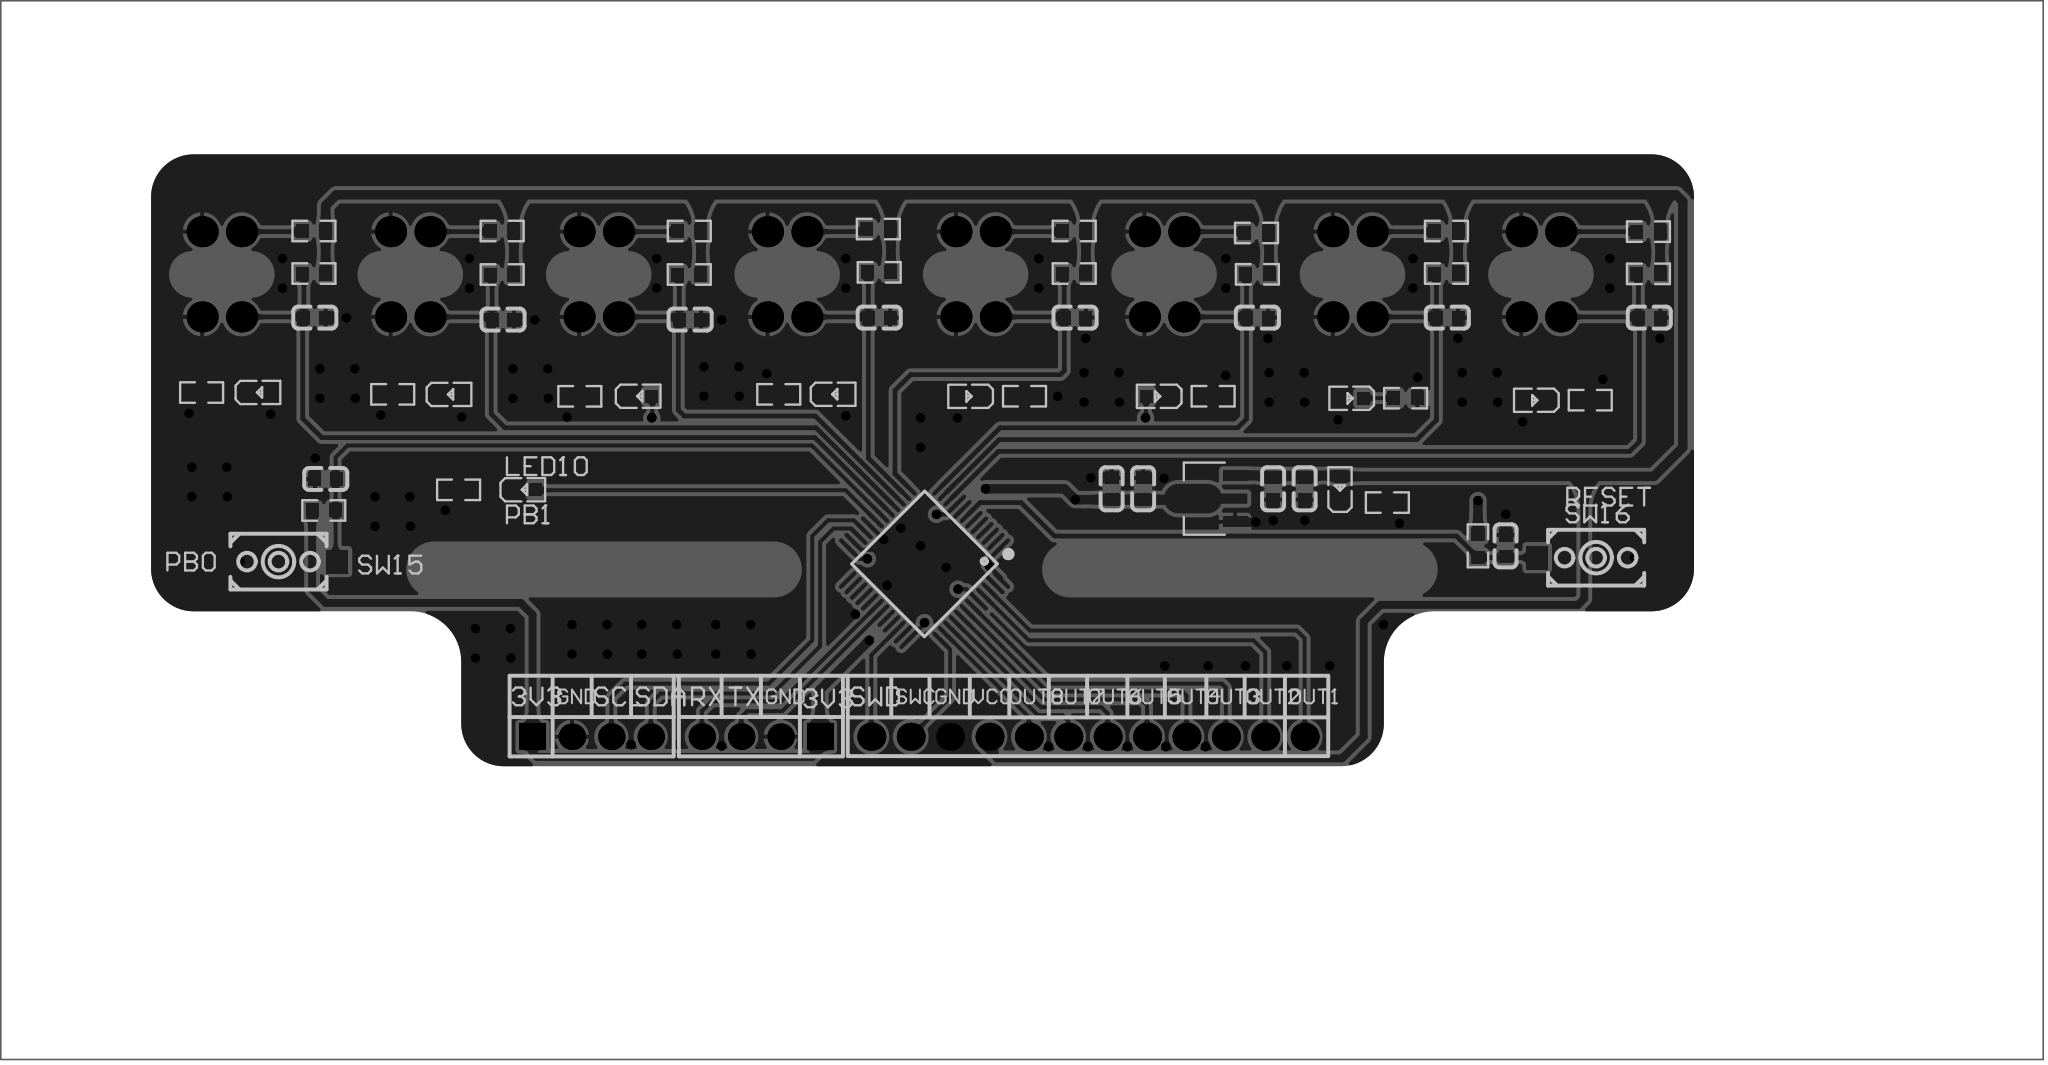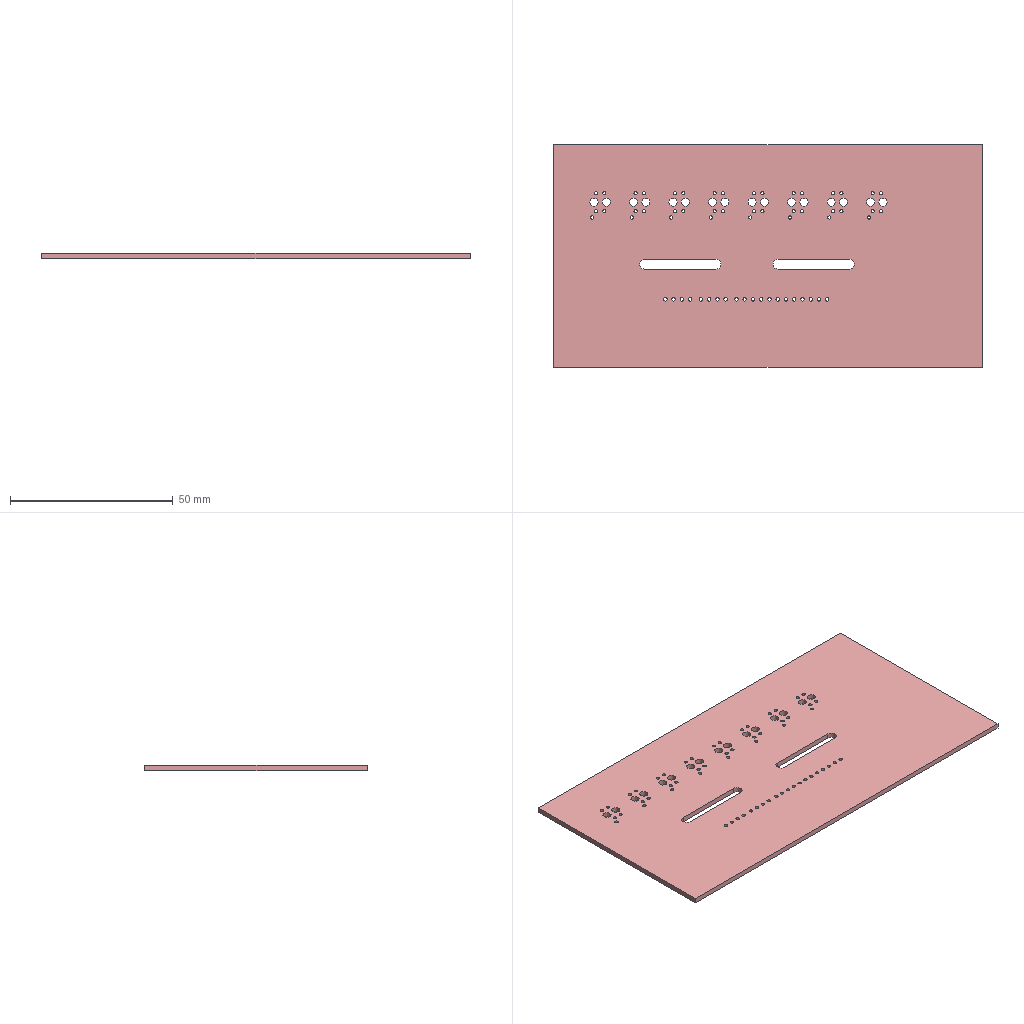Circuit board layout | Altium Designer | box 131.7 x 68.3 x 1.6 mm
Layer stack:
# Altium Designer layer stack of  (unit mm; dielectric type: 0 none, 1 core, 2 prepreg, 3 surface material)
index,name,kind,layer,copper_thickness_mm,dielectric_type,dielectric_thickness_mm,dielectric_material,dielectric_constant
0,Top Paste Mask Layer,other,,,,,,
1,Top Silkscreen Layer,other,,,,,,
2,Top Solder Mask Layer,dielectric,,,3,0.01,,3.3
3,Top Layer,copper,Top Layer,0.035,,,,
4,Dielectric1,dielectric,,,3,1.51,FR4,4.5
5,Bottom Layer,copper,Bottom Layer,0.035,,,,
6,Bottom Solder Mask Layer,dielectric,,,3,0.01,,3.3
7,Bottom Silkscreen Layer,other,,,,,,
8,Bottom Paste Mask Layer,other,,,,,,
# drill layer pairs: low layer,high layer
drill_pair,Top Layer,Bottom Layer
Part placement:
Designator,Comment,Layer,Footprint,Center-X(mm),Center-Y(mm),Rotation
CGQ1,TCRT5000L,BottomLayer,OPTO-TH_TCRT5000L,169.164,120.523,90
CGQ2,TCRT5000L,BottomLayer,OPTO-TH_TCRT5000L,157.013,120.523,90
CGQ3,TCRT5000L,BottomLayer,OPTO-TH_TCRT5000L,144.862,120.523,90
CGQ4,TCRT5000L,BottomLayer,OPTO-TH_TCRT5000L,132.711,120.523,90
CGQ5,TCRT5000L,BottomLayer,OPTO-TH_TCRT5000L,120.559,120.523,90
CGQ6,TCRT5000L,BottomLayer,OPTO-TH_TCRT5000L,108.408,120.523,90
CGQ7,TCRT5000L,BottomLayer,OPTO-TH_TCRT5000L,96.257,120.523,90
CGQ8,TCRT5000L,BottomLayer,OPTO-TH_TCRT5000L,84.106,120.523,90
H1,,TopLayer,HDR-TH_12P-P2.54-V-F,139.954,90.678,180
H2,,TopLayer,HDR-TH_4P-P2.54-V-F,107.95,90.678,0
H3,,TopLayer,HDR-TH_4P-P2.54-V-F,118.864,90.683,180
LED1,NCD0603R1,TopLayer,LED0603-RD_RED,168.815,112.4,180
LED2,NCD0603R1,TopLayer,LED0603-RD_RED,156.91,112.527,180
LED3,NCD0603R1,TopLayer,LED0603-RD_RED,144.496,112.654,180
LED4,NCD0603R1,TopLayer,LED0603-RD_RED,132.336,112.654,180
LED5,NCD0603R1,TopLayer,LED0603-RD_RED,123.571,112.776,0
LED6,NCD0603R1,TopLayer,LED0603-RD_RED,110.998,112.649,0
LED7,NCD0603R1,TopLayer,LED0603-RD_RED,98.802,112.765,0
LED8,NCD0603R1,TopLayer,LED0603-RD_RED,86.483,112.892,0
LED9,NCD0603R1,TopLayer,LED0603-RD_RED,156.21,106.68,90
LED10,NCD0603R1,TopLayer,LED0603-RD_RED,103.561,106.613,0
R1,10kΩ,TopLayer,R0603,176.093,120.553,0
R2,1kΩ,TopLayer,R0603,176.093,123.277,0
R3,1kΩ,TopLayer,R0603,172.341,112.4,0
R4,10kΩ,TopLayer,R0603,163.068,120.573,0
R5,1kΩ,TopLayer,R0603,163.068,123.317,0
R6,1kΩ,TopLayer,R0603,160.435,112.527,0
R7,10kΩ,TopLayer,R0603,150.876,120.523,0
R8,1kΩ,TopLayer,R0603,150.82,123.19,0
R9,1kΩ,TopLayer,R0603,148.022,112.654,0
R10,10kΩ,TopLayer,R0603,139.065,120.573,0
R11,1kΩ,TopLayer,R0603,139.065,123.317,0
R12,1kΩ,TopLayer,R0603,135.862,112.654,0
R13,10kΩ,TopLayer,R0603,126.492,120.65,0
R14,1kΩ,TopLayer,R0603,126.436,123.444,0
R15,1kΩ,TopLayer,R0603,120.015,112.776,180
R16,10kΩ,TopLayer,R0603,114.244,120.51,0
R17,1kΩ,TopLayer,R0603,114.244,123.317,0
R18,1kΩ,TopLayer,R0603,107.188,112.649,180
R19,10kΩ,TopLayer,R0603,102.179,120.51,0
R20,1kΩ,TopLayer,R0603,102.179,123.317,0
R21,1kΩ,TopLayer,R0603,95.123,112.776,180
R22,10kΩ,TopLayer,R0603,90.043,120.573,0
R23,1kΩ,TopLayer,R0603,90.043,123.317,0
R24,1kΩ,TopLayer,R0603,82.8,112.892,180
R86,1kΩ,TopLayer,R0603,159.258,105.791,0
R87,1kΩ,TopLayer,R0603,99.37,106.613,180
SW15,K2-1107ST-A4DW-06,TopLayer,KEY-SMD_L6.2-W3.6-LS8.0,87.757,101.981,180
SW16,K2-1107ST-A4DW-06,TopLayer,KEY-SMD_L6.2-W3.6-LS8.0,172.72,102.235,0
U1,STM32F103C8T6,TopLayer,LQFP-48_L7.0-W7.0-P0.50-LS9.0-BL,129.413,101.854,135
U3,CJA1117B-3.3,TopLayer,SOT-89-3_L4.5-W2.5-P1.50-LS4.2-BR,148.277,106.045,0
C11,100nF,BottomLayer,C0603,127.127,102.235,225
C12,100nF,BottomLayer,C0603,129.54,104.521,315
C13,100nF,BottomLayer,C0603,131.953,102.235,315
C14,100nF,BottomLayer,C0603,128.905,99.695,315
C19,100nF,TopLayer,C0603,143.51,106.68,270
C21,100nF,TopLayer,C0603,151.892,106.68,90
C26,10uF,TopLayer,C0603,153.924,106.68,270
C27,10uF,TopLayer,C0603,141.478,106.68,90
C28,100nF,TopLayer,C0603,90.805,107.315,0
C29,100nF,TopLayer,C0603,166.878,102.997,270
C30,100nF,TopLayer,C0603,176.149,117.729,0
C31,100nF,TopLayer,C0603,163.124,117.729,0
C32,100nF,TopLayer,C0603,150.876,117.729,0
C33,100nF,TopLayer,C0603,139.121,117.729,0
C34,100nF,TopLayer,C0603,126.492,117.729,0
C35,100nF,TopLayer,C0603,114.3,117.602,0
C36,100nF,TopLayer,C0603,102.235,117.602,0
C37,100nF,TopLayer,C0603,90.099,117.729,0
R84,10K,TopLayer,R0603,90.678,105.283,180
R85,10K,TopLayer,R0603,165.1,102.997,90
R83,1kΩ,BottomLayer,R0603,130.175,101.092,315
Pad and via stacks:
# Altium Designer via and pad stacks of  (unit mm). Each distinct definition once, with the count of objects using it.
# via: kind,start_layer,end_layer,hole_mm,diameter_mm,mode(0 simple;1 top-mid-bottom;2 full stack),diameter_per_layer,count,example_net
# pad: kind,layer,hole_mm,hole_type(0 round;1 square;2 slot),plating,top_size,top_shape(1 round;2 rect;3 octagon;9 rounded rect),mid_size,bottom_size,mode,footprint,size_per_layer,count,example
pad,Multi-Layer,1,0,plated,2x2,1,2x2,2x2,0,OPTO-TH_TCRT5000L,,32,CGQ1.1
pad,Multi-Layer,1.05,0,plated,1.8x1.8,1,1.8x1.8,1.8x1.8,0,HDR-TH_12P-P2.54-V-F,,12,H1.1
pad,Multi-Layer,1.1,0,plated,1.7x1.7,2,1.7x1.7,1.7x1.7,0,HDR-TH_4P-P2.54-V-F,,2,H2.1
pad,Multi-Layer,1.1,0,plated,1.7x1.7,1,1.7x1.7,1.7x1.7,0,HDR-TH_4P-P2.54-V-F,,6,H2.2
pad,Top Layer,0,0,plated,0.8x0.8,2,0.8x0.8,0.8x0.8,0,LED0603-RD_RED,,20,LED1.1
pad,Top Layer,0,0,plated,0.8065x0.864,2,0.8065x0.864,0.8065x0.864,0,R0603,,56,R1.2
pad,Top Layer,0,0,plated,1.5x1.4,2,1.5x1.4,1.5x1.4,0,KEY-SMD_L6.2-W3.6-LS8.0,,4,SW15.1
pad,Top Layer,0,0,plated,0.27x1.5,1,0.27x1.5,0.27x1.5,0,LQFP-48_L7.0-W7.0-P0.50-LS9.0-BL,,24,U1.1
pad,Top Layer,0,0,plated,1.5x0.27,1,1.5x0.27,1.5x0.27,0,LQFP-48_L7.0-W7.0-P0.50-LS9.0-BL,,24,U1.13
pad,Top Layer,0,0,plated,1.575x0.672,2,1.575x0.672,1.575x0.672,0,SOT-89-3_L4.5-W2.5-P1.50-LS4.2-BR,,2,U3.1
pad,Top Layer,0,0,plated,0.95x0.95,1,0.95x0.95,0.95x0.95,0,SOT-89-3_L4.5-W2.5-P1.50-LS4.2-BR,,1,U3.2
pad,Top Layer,0,0,plated,0.8x0.9,2,0.8x0.9,0.8x0.9,0,C0603,,28,C19.2
pad,Bottom Layer,0,0,plated,0.8x0.9,2,0.8x0.9,0.8x0.9,0,C0603,,8,C11.2
pad,Bottom Layer,0,0,plated,0.8065x0.864,2,0.8065x0.864,0.8065x0.864,0,R0603,,2,R83.2
via,Top Layer,Bottom Layer,0.3048,0.61,0,,129,3V3
Copper pours:
name,layer,net,type(0 solid;1 hatched;2 none)
Bottom Layer-GND,Bottom Layer,GND,0
Top Layer-GND,Top Layer,GND,0